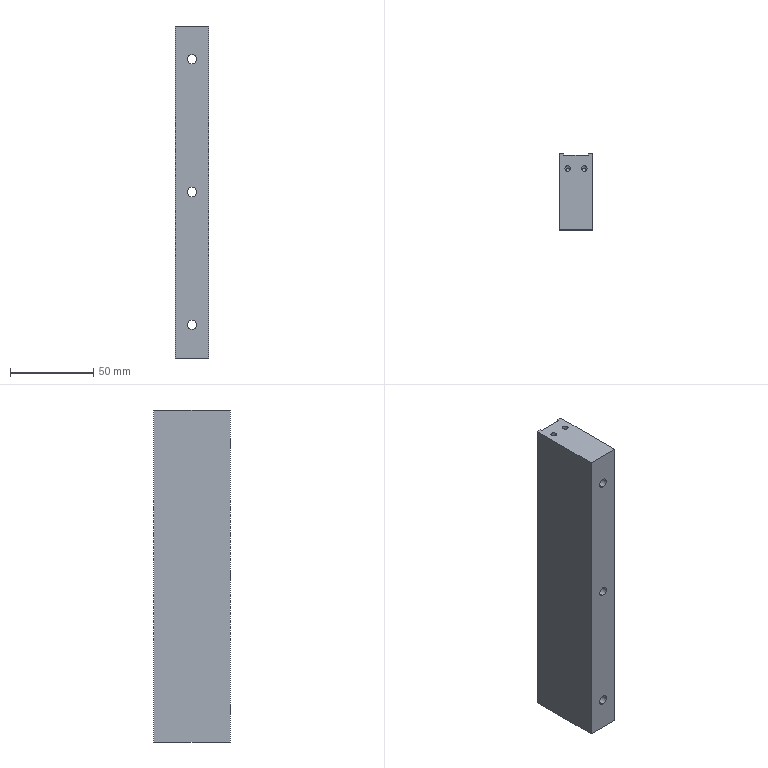Part | STEP file | PN_0080 transport section guide rail pad block B | 1 solid | 57 faces | box 20 x 46 x 200 mm | volume 172286 mm3 | cylinder 28 | cone 16 | plane 13 | commonest cylinder face diameters 2.5 x8 3.3 x8 5.5 x6 10 x6